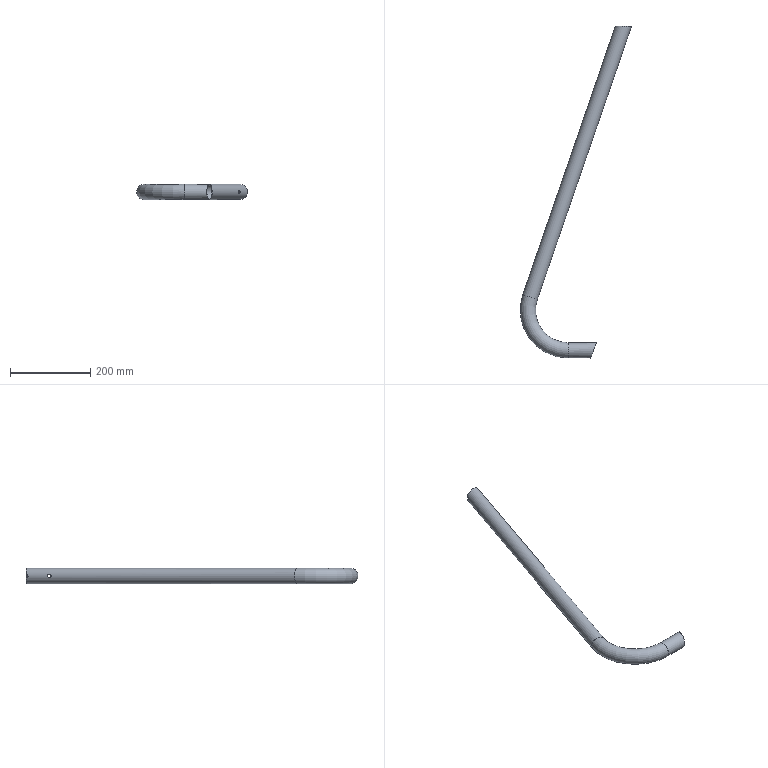Part | STEP file | 6101401 | 1 solid | 11 faces | box 276.919 x 826.178 x 38.1 mm | volume 166528 mm3 | cylinder 7 | torus 2 | plane 2 | commonest cylinder face diameters 9 x2 35.1 x2 38.1 x2 10 x1